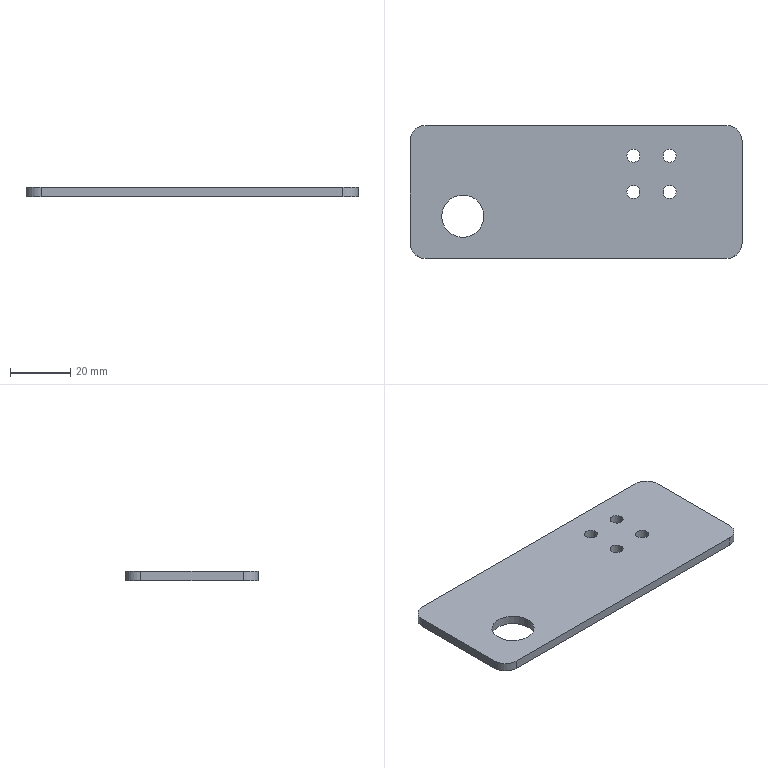Part | SolidWorks | features Fillet 2, Cut 1, Extrusion 1, ICE 1 | 1 solid | 20 faces | box 110 x 44 x 3 mm | volume 13820 mm3 | cylinder 14 | plane 6 | commonest cylinder face diameters 4.3 x8 10 x4 14 x2
STEP:
#1=CARTESIAN_POINT('',(-69.5,-8.,0.));
#2=VERTEX_POINT('',#1);
#3=CARTESIAN_POINT('',(-55.5,-8.,0.));
#4=VERTEX_POINT('',#3);
#5=CARTESIAN_POINT('',(-62.5,-8.,0.));
#6=DIRECTION('',(0.,0.,1.));
#7=DIRECTION('',(1.,0.,0.));
#8=AXIS2_PLACEMENT_3D('',#5,#6,#7);
#9=CIRCLE('',#8,7.);
#10=EDGE_CURVE('',#2,#4,#9,.T.);
#11=ORIENTED_EDGE('',*,*,#10,.F.);
#12=CARTESIAN_POINT('',(-69.5,-8.,3.));
#13=VERTEX_POINT('',#12);
#14=CARTESIAN_POINT('',(-69.5,-8.,0.));
#15=DIRECTION('',(0.,0.,1.));
#16=VECTOR('',#15,1000.);
#17=LINE('',#14,#16);
#18=EDGE_CURVE('',#2,#13,#17,.T.);
#19=ORIENTED_EDGE('',*,*,#18,.T.);
#20=CARTESIAN_POINT('',(-55.5,-8.,3.));
#21=VERTEX_POINT('',#20);
#22=CARTESIAN_POINT('',(-62.5,-8.,3.));
#23=DIRECTION('',(0.,0.,1.));
#24=DIRECTION('',(1.,0.,0.));
#25=AXIS2_PLACEMENT_3D('',#22,#23,#24);
#26=CIRCLE('',#25,7.);
#27=EDGE_CURVE('',#13,#21,#26,.T.);
#28=ORIENTED_EDGE('',*,*,#27,.T.);
#29=CARTESIAN_POINT('',(-55.5,-8.,0.));
#30=DIRECTION('',(0.,0.,1.));
#31=VECTOR('',#30,1000.);
#32=LINE('',#29,#31);
#33=EDGE_CURVE('',#4,#21,#32,.T.);
#34=ORIENTED_EDGE('',*,*,#33,.F.);
#35=EDGE_LOOP('',(#11,#19,#28,#34));
#36=FACE_OUTER_BOUND('',#35,.T.);
#37=CARTESIAN_POINT('',(-62.5,-8.,0.));
#38=DIRECTION('',(0.,0.,1.));
#39=DIRECTION('',(1.,0.,0.));
#40=AXIS2_PLACEMENT_3D('',#37,#38,#39);
#41=CYLINDRICAL_SURFACE('',#40,7.);
#42=ADVANCED_FACE('',(#36),#41,.F.);
#43=CARTESIAN_POINT('',(-8.15,0.,0.));
#44=VERTEX_POINT('',#43);
#45=CARTESIAN_POINT('',(-3.85,0.,0.));
#46=VERTEX_POINT('',#45);
#47=CARTESIAN_POINT('',(-6.,0.,0.));
#48=DIRECTION('',(0.,0.,1.));
#49=DIRECTION('',(1.,0.,0.));
#50=AXIS2_PLACEMENT_3D('',#47,#48,#49);
#51=CIRCLE('',#50,2.15);
#52=EDGE_CURVE('',#44,#46,#51,.T.);
#53=ORIENTED_EDGE('',*,*,#52,.F.);
#54=CARTESIAN_POINT('',(-8.15,0.,3.));
#55=VERTEX_POINT('',#54);
#56=CARTESIAN_POINT('',(-8.15,0.,0.));
#57=DIRECTION('',(0.,0.,1.));
#58=VECTOR('',#57,1000.);
#59=LINE('',#56,#58);
#60=EDGE_CURVE('',#44,#55,#59,.T.);
#61=ORIENTED_EDGE('',*,*,#60,.T.);
#62=CARTESIAN_POINT('',(-3.85,0.,3.));
#63=VERTEX_POINT('',#62);
#64=CARTESIAN_POINT('',(-6.,0.,3.));
#65=DIRECTION('',(0.,0.,1.));
#66=DIRECTION('',(1.,0.,0.));
#67=AXIS2_PLACEMENT_3D('',#64,#65,#66);
#68=CIRCLE('',#67,2.15);
#69=EDGE_CURVE('',#55,#63,#68,.T.);
#70=ORIENTED_EDGE('',*,*,#69,.T.);
#71=CARTESIAN_POINT('',(-3.85,0.,0.));
#72=DIRECTION('',(0.,0.,1.));
#73=VECTOR('',#72,1000.);
#74=LINE('',#71,#73);
#75=EDGE_CURVE('',#46,#63,#74,.T.);
#76=ORIENTED_EDGE('',*,*,#75,.F.);
#77=EDGE_LOOP('',(#53,#61,#70,#76));
#78=FACE_OUTER_BOUND('',#77,.T.);
#79=CARTESIAN_POINT('',(-6.,0.,0.));
#80=DIRECTION('',(0.,0.,1.));
#81=DIRECTION('',(1.,0.,0.));
#82=AXIS2_PLACEMENT_3D('',#79,#80,#81);
#83=CYLINDRICAL_SURFACE('',#82,2.15);
#84=ADVANCED_FACE('',(#78),#83,.F.);
#85=CARTESIAN_POINT('',(-8.15,12.,0.));
#86=VERTEX_POINT('',#85);
#87=CARTESIAN_POINT('',(-3.85,12.,0.));
#88=VERTEX_POINT('',#87);
#89=CARTESIAN_POINT('',(-6.,12.,0.));
#90=DIRECTION('',(0.,0.,1.));
#91=DIRECTION('',(1.,0.,0.));
#92=AXIS2_PLACEMENT_3D('',#89,#90,#91);
#93=CIRCLE('',#92,2.15);
#94=EDGE_CURVE('',#86,#88,#93,.T.);
#95=ORIENTED_EDGE('',*,*,#94,.F.);
#96=CARTESIAN_POINT('',(-8.15,12.,3.));
#97=VERTEX_POINT('',#96);
#98=CARTESIAN_POINT('',(-8.15,12.,0.));
#99=DIRECTION('',(0.,0.,1.));
#100=VECTOR('',#99,1000.);
#101=LINE('',#98,#100);
#102=EDGE_CURVE('',#86,#97,#101,.T.);
#103=ORIENTED_EDGE('',*,*,#102,.T.);
#104=CARTESIAN_POINT('',(-3.85,12.,3.));
#105=VERTEX_POINT('',#104);
#106=CARTESIAN_POINT('',(-6.,12.,3.));
#107=DIRECTION('',(0.,0.,1.));
#108=DIRECTION('',(1.,0.,0.));
#109=AXIS2_PLACEMENT_3D('',#106,#107,#108);
#110=CIRCLE('',#109,2.15);
#111=EDGE_CURVE('',#97,#105,#110,.T.);
#112=ORIENTED_EDGE('',*,*,#111,.T.);
#113=CARTESIAN_POINT('',(-3.85,12.,0.));
#114=DIRECTION('',(0.,0.,1.));
#115=VECTOR('',#114,1000.);
#116=LINE('',#113,#115);
#117=EDGE_CURVE('',#88,#105,#116,.T.);
#118=ORIENTED_EDGE('',*,*,#117,.F.);
#119=EDGE_LOOP('',(#95,#103,#112,#118));
#120=FACE_OUTER_BOUND('',#119,.T.);
#121=CARTESIAN_POINT('',(-6.,12.,0.));
#122=DIRECTION('',(0.,0.,1.));
#123=DIRECTION('',(1.,0.,0.));
#124=AXIS2_PLACEMENT_3D('',#121,#122,#123);
#125=CYLINDRICAL_SURFACE('',#124,2.15);
#126=ADVANCED_FACE('',(#120),#125,.F.);
#127=CARTESIAN_POINT('',(3.85,12.,0.));
#128=VERTEX_POINT('',#127);
#129=CARTESIAN_POINT('',(8.15,12.,0.));
#130=VERTEX_POINT('',#129);
#131=CARTESIAN_POINT('',(6.,12.,0.));
#132=DIRECTION('',(0.,0.,1.));
#133=DIRECTION('',(1.,0.,0.));
#134=AXIS2_PLACEMENT_3D('',#131,#132,#133);
#135=CIRCLE('',#134,2.15);
#136=EDGE_CURVE('',#128,#130,#135,.T.);
#137=ORIENTED_EDGE('',*,*,#136,.F.);
#138=CARTESIAN_POINT('',(3.85,12.,3.));
#139=VERTEX_POINT('',#138);
#140=CARTESIAN_POINT('',(3.85,12.,0.));
#141=DIRECTION('',(0.,0.,1.));
#142=VECTOR('',#141,1000.);
#143=LINE('',#140,#142);
#144=EDGE_CURVE('',#128,#139,#143,.T.);
#145=ORIENTED_EDGE('',*,*,#144,.T.);
#146=CARTESIAN_POINT('',(8.15,12.,3.));
#147=VERTEX_POINT('',#146);
#148=CARTESIAN_POINT('',(6.,12.,3.));
#149=DIRECTION('',(0.,0.,1.));
#150=DIRECTION('',(1.,0.,0.));
#151=AXIS2_PLACEMENT_3D('',#148,#149,#150);
#152=CIRCLE('',#151,2.15);
#153=EDGE_CURVE('',#139,#147,#152,.T.);
#154=ORIENTED_EDGE('',*,*,#153,.T.);
#155=CARTESIAN_POINT('',(8.15,12.,0.));
#156=DIRECTION('',(0.,0.,1.));
#157=VECTOR('',#156,1000.);
#158=LINE('',#155,#157);
#159=EDGE_CURVE('',#130,#147,#158,.T.);
#160=ORIENTED_EDGE('',*,*,#159,.F.);
#161=EDGE_LOOP('',(#137,#145,#154,#160));
#162=FACE_OUTER_BOUND('',#161,.T.);
#163=CARTESIAN_POINT('',(6.,12.,0.));
#164=DIRECTION('',(0.,0.,1.));
#165=DIRECTION('',(1.,0.,0.));
#166=AXIS2_PLACEMENT_3D('',#163,#164,#165);
#167=CYLINDRICAL_SURFACE('',#166,2.15);
#168=ADVANCED_FACE('',(#162),#167,.F.);
#169=CARTESIAN_POINT('',(3.85,0.,0.));
#170=VERTEX_POINT('',#169);
#171=CARTESIAN_POINT('',(8.15,0.,0.));
#172=VERTEX_POINT('',#171);
#173=CARTESIAN_POINT('',(6.,0.,0.));
#174=DIRECTION('',(0.,0.,1.));
#175=DIRECTION('',(1.,0.,0.));
#176=AXIS2_PLACEMENT_3D('',#173,#174,#175);
#177=CIRCLE('',#176,2.15);
#178=EDGE_CURVE('',#170,#172,#177,.T.);
#179=ORIENTED_EDGE('',*,*,#178,.F.);
#180=CARTESIAN_POINT('',(3.85,0.,3.));
#181=VERTEX_POINT('',#180);
#182=CARTESIAN_POINT('',(3.85,0.,0.));
#183=DIRECTION('',(0.,0.,1.));
#184=VECTOR('',#183,1000.);
#185=LINE('',#182,#184);
#186=EDGE_CURVE('',#170,#181,#185,.T.);
#187=ORIENTED_EDGE('',*,*,#186,.T.);
#188=CARTESIAN_POINT('',(8.15,0.,3.));
#189=VERTEX_POINT('',#188);
#190=CARTESIAN_POINT('',(6.,0.,3.));
#191=DIRECTION('',(0.,0.,1.));
#192=DIRECTION('',(1.,0.,0.));
#193=AXIS2_PLACEMENT_3D('',#190,#191,#192);
#194=CIRCLE('',#193,2.15);
#195=EDGE_CURVE('',#181,#189,#194,.T.);
#196=ORIENTED_EDGE('',*,*,#195,.T.);
#197=CARTESIAN_POINT('',(8.15,0.,0.));
#198=DIRECTION('',(0.,0.,1.));
#199=VECTOR('',#198,1000.);
#200=LINE('',#197,#199);
#201=EDGE_CURVE('',#172,#189,#200,.T.);
#202=ORIENTED_EDGE('',*,*,#201,.F.);
#203=EDGE_LOOP('',(#179,#187,#196,#202));
#204=FACE_OUTER_BOUND('',#203,.T.);
#205=CARTESIAN_POINT('',(6.,0.,0.));
#206=DIRECTION('',(0.,0.,1.));
#207=DIRECTION('',(1.,0.,0.));
#208=AXIS2_PLACEMENT_3D('',#205,#206,#207);
#209=CYLINDRICAL_SURFACE('',#208,2.15);
#210=ADVANCED_FACE('',(#204),#209,.F.);
#211=CARTESIAN_POINT('',(25.,22.,3.));
#212=VERTEX_POINT('',#211);
#213=CARTESIAN_POINT('',(-75.,22.,3.));
#214=VERTEX_POINT('',#213);
#215=CARTESIAN_POINT('',(-80.,22.,3.));
#216=DIRECTION('',(-1.,0.,0.));
#217=VECTOR('',#216,1000.);
#218=LINE('',#215,#217);
#219=EDGE_CURVE('',#212,#214,#218,.T.);
#220=ORIENTED_EDGE('',*,*,#219,.F.);
#221=CARTESIAN_POINT('',(25.,22.,0.));
#222=VERTEX_POINT('',#221);
#223=CARTESIAN_POINT('',(25.,22.,3.));
#224=DIRECTION('',(0.,0.,-1.));
#225=VECTOR('',#224,1000.);
#226=LINE('',#223,#225);
#227=EDGE_CURVE('',#212,#222,#226,.T.);
#228=ORIENTED_EDGE('',*,*,#227,.T.);
#229=CARTESIAN_POINT('',(-75.,22.,0.));
#230=VERTEX_POINT('',#229);
#231=CARTESIAN_POINT('',(-80.,22.,0.));
#232=DIRECTION('',(-1.,0.,0.));
#233=VECTOR('',#232,1000.);
#234=LINE('',#231,#233);
#235=EDGE_CURVE('',#222,#230,#234,.T.);
#236=ORIENTED_EDGE('',*,*,#235,.T.);
#237=CARTESIAN_POINT('',(-75.,22.,3.));
#238=DIRECTION('',(0.,0.,1.));
#239=VECTOR('',#238,1000.);
#240=LINE('',#237,#239);
#241=EDGE_CURVE('',#230,#214,#240,.T.);
#242=ORIENTED_EDGE('',*,*,#241,.T.);
#243=EDGE_LOOP('',(#220,#228,#236,#242));
#244=FACE_OUTER_BOUND('',#243,.T.);
#245=CARTESIAN_POINT('',(-80.,22.,3.));
#246=DIRECTION('',(0.,-1.,0.));
#247=DIRECTION('',(0.,0.,-1.));
#248=AXIS2_PLACEMENT_3D('',#245,#246,#247);
#249=PLANE('',#248);
#250=ADVANCED_FACE('',(#244),#249,.F.);
#251=CARTESIAN_POINT('',(-80.,17.,3.));
#252=VERTEX_POINT('',#251);
#253=CARTESIAN_POINT('',(-80.,-17.,3.));
#254=VERTEX_POINT('',#253);
#255=CARTESIAN_POINT('',(-80.,22.,3.));
#256=DIRECTION('',(0.,-1.,0.));
#257=VECTOR('',#256,1000.);
#258=LINE('',#255,#257);
#259=EDGE_CURVE('',#252,#254,#258,.T.);
#260=ORIENTED_EDGE('',*,*,#259,.F.);
#261=CARTESIAN_POINT('',(-80.,17.,0.));
#262=VERTEX_POINT('',#261);
#263=CARTESIAN_POINT('',(-80.,17.,3.));
#264=DIRECTION('',(0.,0.,-1.));
#265=VECTOR('',#264,1000.);
#266=LINE('',#263,#265);
#267=EDGE_CURVE('',#252,#262,#266,.T.);
#268=ORIENTED_EDGE('',*,*,#267,.T.);
#269=CARTESIAN_POINT('',(-80.,-17.,0.));
#270=VERTEX_POINT('',#269);
#271=CARTESIAN_POINT('',(-80.,22.,0.));
#272=DIRECTION('',(0.,-1.,0.));
#273=VECTOR('',#272,1000.);
#274=LINE('',#271,#273);
#275=EDGE_CURVE('',#262,#270,#274,.T.);
#276=ORIENTED_EDGE('',*,*,#275,.T.);
#277=CARTESIAN_POINT('',(-80.,-17.,3.));
#278=DIRECTION('',(0.,0.,1.));
#279=VECTOR('',#278,1000.);
#280=LINE('',#277,#279);
#281=EDGE_CURVE('',#270,#254,#280,.T.);
#282=ORIENTED_EDGE('',*,*,#281,.T.);
#283=EDGE_LOOP('',(#260,#268,#276,#282));
#284=FACE_OUTER_BOUND('',#283,.T.);
#285=CARTESIAN_POINT('',(-80.,22.,3.));
#286=DIRECTION('',(1.,0.,0.));
#287=DIRECTION('',(0.,0.,-1.));
#288=AXIS2_PLACEMENT_3D('',#285,#286,#287);
#289=PLANE('',#288);
#290=ADVANCED_FACE('',(#284),#289,.F.);
#291=CARTESIAN_POINT('',(-75.,-22.,0.));
#292=VERTEX_POINT('',#291);
#293=CARTESIAN_POINT('',(25.,-22.,0.));
#294=VERTEX_POINT('',#293);
#295=CARTESIAN_POINT('',(-80.,-22.,0.));
#296=DIRECTION('',(1.,0.,0.));
#297=VECTOR('',#296,1000.);
#298=LINE('',#295,#297);
#299=EDGE_CURVE('',#292,#294,#298,.T.);
#300=ORIENTED_EDGE('',*,*,#299,.T.);
#301=CARTESIAN_POINT('',(25.,-22.,3.));
#302=VERTEX_POINT('',#301);
#303=CARTESIAN_POINT('',(25.,-22.,3.));
#304=DIRECTION('',(0.,0.,1.));
#305=VECTOR('',#304,1000.);
#306=LINE('',#303,#305);
#307=EDGE_CURVE('',#294,#302,#306,.T.);
#308=ORIENTED_EDGE('',*,*,#307,.T.);
#309=CARTESIAN_POINT('',(-75.,-22.,3.));
#310=VERTEX_POINT('',#309);
#311=CARTESIAN_POINT('',(-80.,-22.,3.));
#312=DIRECTION('',(1.,0.,0.));
#313=VECTOR('',#312,1000.);
#314=LINE('',#311,#313);
#315=EDGE_CURVE('',#310,#302,#314,.T.);
#316=ORIENTED_EDGE('',*,*,#315,.F.);
#317=CARTESIAN_POINT('',(-75.,-22.,3.));
#318=DIRECTION('',(0.,0.,-1.));
#319=VECTOR('',#318,1000.);
#320=LINE('',#317,#319);
#321=EDGE_CURVE('',#310,#292,#320,.T.);
#322=ORIENTED_EDGE('',*,*,#321,.T.);
#323=EDGE_LOOP('',(#300,#308,#316,#322));
#324=FACE_OUTER_BOUND('',#323,.T.);
#325=CARTESIAN_POINT('',(-80.,-22.,3.));
#326=DIRECTION('',(0.,1.,0.));
#327=DIRECTION('',(0.,0.,1.));
#328=AXIS2_PLACEMENT_3D('',#325,#326,#327);
#329=PLANE('',#328);
#330=ADVANCED_FACE('',(#324),#329,.F.);
#331=ORIENTED_EDGE('',*,*,#315,.T.);
#332=CARTESIAN_POINT('',(30.,-17.,3.));
#333=VERTEX_POINT('',#332);
#334=CARTESIAN_POINT('',(25.,-17.,3.));
#335=DIRECTION('',(0.,0.,1.));
#336=DIRECTION('',(1.,0.,0.));
#337=AXIS2_PLACEMENT_3D('',#334,#335,#336);
#338=CIRCLE('',#337,5.);
#339=EDGE_CURVE('',#302,#333,#338,.T.);
#340=ORIENTED_EDGE('',*,*,#339,.T.);
#341=CARTESIAN_POINT('',(30.,17.,3.));
#342=VERTEX_POINT('',#341);
#343=CARTESIAN_POINT('',(30.,-36.164,3.));
#344=DIRECTION('',(0.,-1.,0.));
#345=VECTOR('',#344,1000.);
#346=LINE('',#343,#345);
#347=EDGE_CURVE('',#342,#333,#346,.T.);
#348=ORIENTED_EDGE('',*,*,#347,.F.);
#349=CARTESIAN_POINT('',(25.,17.,3.));
#350=DIRECTION('',(0.,0.,1.));
#351=DIRECTION('',(1.,0.,0.));
#352=AXIS2_PLACEMENT_3D('',#349,#350,#351);
#353=CIRCLE('',#352,5.);
#354=EDGE_CURVE('',#342,#212,#353,.T.);
#355=ORIENTED_EDGE('',*,*,#354,.T.);
#356=ORIENTED_EDGE('',*,*,#219,.T.);
#357=CARTESIAN_POINT('',(-75.,17.,3.));
#358=DIRECTION('',(0.,0.,1.));
#359=DIRECTION('',(1.,0.,0.));
#360=AXIS2_PLACEMENT_3D('',#357,#358,#359);
#361=CIRCLE('',#360,5.);
#362=EDGE_CURVE('',#214,#252,#361,.T.);
#363=ORIENTED_EDGE('',*,*,#362,.T.);
#364=ORIENTED_EDGE('',*,*,#259,.T.);
#365=CARTESIAN_POINT('',(-75.,-17.,3.));
#366=DIRECTION('',(0.,0.,1.));
#367=DIRECTION('',(1.,0.,0.));
#368=AXIS2_PLACEMENT_3D('',#365,#366,#367);
#369=CIRCLE('',#368,5.);
#370=EDGE_CURVE('',#254,#310,#369,.T.);
#371=ORIENTED_EDGE('',*,*,#370,.T.);
#372=EDGE_LOOP('',(#331,#340,#348,#355,#356,#363,#364,#371));
#373=FACE_OUTER_BOUND('',#372,.T.);
#374=CARTESIAN_POINT('',(-62.5,-8.,3.));
#375=DIRECTION('',(0.,0.,1.));
#376=DIRECTION('',(1.,0.,0.));
#377=AXIS2_PLACEMENT_3D('',#374,#375,#376);
#378=CIRCLE('',#377,7.);
#379=EDGE_CURVE('',#21,#13,#378,.T.);
#380=ORIENTED_EDGE('',*,*,#379,.F.);
#381=ORIENTED_EDGE('',*,*,#27,.F.);
#382=EDGE_LOOP('',(#380,#381));
#383=FACE_BOUND('',#382,.T.);
#384=CARTESIAN_POINT('',(-6.,0.,3.));
#385=DIRECTION('',(0.,0.,1.));
#386=DIRECTION('',(1.,0.,0.));
#387=AXIS2_PLACEMENT_3D('',#384,#385,#386);
#388=CIRCLE('',#387,2.15);
#389=EDGE_CURVE('',#63,#55,#388,.T.);
#390=ORIENTED_EDGE('',*,*,#389,.F.);
#391=ORIENTED_EDGE('',*,*,#69,.F.);
#392=EDGE_LOOP('',(#390,#391));
#393=FACE_BOUND('',#392,.T.);
#394=CARTESIAN_POINT('',(-6.,12.,3.));
#395=DIRECTION('',(0.,0.,1.));
#396=DIRECTION('',(1.,0.,0.));
#397=AXIS2_PLACEMENT_3D('',#394,#395,#396);
#398=CIRCLE('',#397,2.15);
#399=EDGE_CURVE('',#105,#97,#398,.T.);
#400=ORIENTED_EDGE('',*,*,#399,.F.);
#401=ORIENTED_EDGE('',*,*,#111,.F.);
#402=EDGE_LOOP('',(#400,#401));
#403=FACE_BOUND('',#402,.T.);
#404=CARTESIAN_POINT('',(6.,12.,3.));
#405=DIRECTION('',(0.,0.,1.));
#406=DIRECTION('',(1.,0.,0.));
#407=AXIS2_PLACEMENT_3D('',#404,#405,#406);
#408=CIRCLE('',#407,2.15);
#409=EDGE_CURVE('',#147,#139,#408,.T.);
#410=ORIENTED_EDGE('',*,*,#409,.F.);
#411=ORIENTED_EDGE('',*,*,#153,.F.);
#412=EDGE_LOOP('',(#410,#411));
#413=FACE_BOUND('',#412,.T.);
#414=CARTESIAN_POINT('',(6.,0.,3.));
#415=DIRECTION('',(0.,0.,1.));
#416=DIRECTION('',(1.,0.,0.));
#417=AXIS2_PLACEMENT_3D('',#414,#415,#416);
#418=CIRCLE('',#417,2.15);
#419=EDGE_CURVE('',#189,#181,#418,.T.);
#420=ORIENTED_EDGE('',*,*,#419,.F.);
#421=ORIENTED_EDGE('',*,*,#195,.F.);
#422=EDGE_LOOP('',(#420,#421));
#423=FACE_BOUND('',#422,.T.);
#424=CARTESIAN_POINT('',(0.,0.,3.));
#425=DIRECTION('',(0.,0.,1.));
#426=DIRECTION('',(1.,0.,0.));
#427=AXIS2_PLACEMENT_3D('',#424,#425,#426);
#428=PLANE('',#427);
#429=ADVANCED_FACE('',(#373,#383,#393,#403,#413,#423),#428,.T.);
#430=CARTESIAN_POINT('',(-62.5,-8.,0.));
#431=DIRECTION('',(0.,0.,1.));
#432=DIRECTION('',(1.,0.,0.));
#433=AXIS2_PLACEMENT_3D('',#430,#431,#432);
#434=CIRCLE('',#433,7.);
#435=EDGE_CURVE('',#4,#2,#434,.T.);
#436=ORIENTED_EDGE('',*,*,#435,.T.);
#437=ORIENTED_EDGE('',*,*,#10,.T.);
#438=EDGE_LOOP('',(#436,#437));
#439=FACE_BOUND('',#438,.T.);
#440=CARTESIAN_POINT('',(-6.,0.,0.));
#441=DIRECTION('',(0.,0.,1.));
#442=DIRECTION('',(1.,0.,0.));
#443=AXIS2_PLACEMENT_3D('',#440,#441,#442);
#444=CIRCLE('',#443,2.15);
#445=EDGE_CURVE('',#46,#44,#444,.T.);
#446=ORIENTED_EDGE('',*,*,#445,.T.);
#447=ORIENTED_EDGE('',*,*,#52,.T.);
#448=EDGE_LOOP('',(#446,#447));
#449=FACE_BOUND('',#448,.T.);
#450=CARTESIAN_POINT('',(-6.,12.,0.));
#451=DIRECTION('',(0.,0.,1.));
#452=DIRECTION('',(1.,0.,0.));
#453=AXIS2_PLACEMENT_3D('',#450,#451,#452);
#454=CIRCLE('',#453,2.15);
#455=EDGE_CURVE('',#88,#86,#454,.T.);
#456=ORIENTED_EDGE('',*,*,#455,.T.);
#457=ORIENTED_EDGE('',*,*,#94,.T.);
#458=EDGE_LOOP('',(#456,#457));
#459=FACE_BOUND('',#458,.T.);
#460=CARTESIAN_POINT('',(6.,12.,0.));
#461=DIRECTION('',(0.,0.,1.));
#462=DIRECTION('',(1.,0.,0.));
#463=AXIS2_PLACEMENT_3D('',#460,#461,#462);
#464=CIRCLE('',#463,2.15);
#465=EDGE_CURVE('',#130,#128,#464,.T.);
#466=ORIENTED_EDGE('',*,*,#465,.T.);
#467=ORIENTED_EDGE('',*,*,#136,.T.);
#468=EDGE_LOOP('',(#466,#467));
#469=FACE_BOUND('',#468,.T.);
#470=CARTESIAN_POINT('',(6.,0.,0.));
#471=DIRECTION('',(0.,0.,1.));
#472=DIRECTION('',(1.,0.,0.));
#473=AXIS2_PLACEMENT_3D('',#470,#471,#472);
#474=CIRCLE('',#473,2.15);
#475=EDGE_CURVE('',#172,#170,#474,.T.);
#476=ORIENTED_EDGE('',*,*,#475,.T.);
#477=ORIENTED_EDGE('',*,*,#178,.T.);
#478=EDGE_LOOP('',(#476,#477));
#479=FACE_BOUND('',#478,.T.);
#480=CARTESIAN_POINT('',(30.,17.,0.));
#481=VERTEX_POINT('',#480);
#482=CARTESIAN_POINT('',(30.,-17.,0.));
#483=VERTEX_POINT('',#482);
#484=CARTESIAN_POINT('',(30.,0.,0.));
#485=DIRECTION('',(0.,-1.,0.));
#486=VECTOR('',#485,1000.);
#487=LINE('',#484,#486);
#488=EDGE_CURVE('',#481,#483,#487,.T.);
#489=ORIENTED_EDGE('',*,*,#488,.T.);
#490=CARTESIAN_POINT('',(25.,-17.,0.));
#491=DIRECTION('',(0.,0.,-1.));
#492=DIRECTION('',(1.,0.,0.));
#493=AXIS2_PLACEMENT_3D('',#490,#491,#492);
#494=CIRCLE('',#493,5.);
#495=EDGE_CURVE('',#483,#294,#494,.T.);
#496=ORIENTED_EDGE('',*,*,#495,.T.);
#497=ORIENTED_EDGE('',*,*,#299,.F.);
#498=CARTESIAN_POINT('',(-75.,-17.,0.));
#499=DIRECTION('',(0.,0.,-1.));
#500=DIRECTION('',(1.,0.,0.));
#501=AXIS2_PLACEMENT_3D('',#498,#499,#500);
#502=CIRCLE('',#501,5.);
#503=EDGE_CURVE('',#292,#270,#502,.T.);
#504=ORIENTED_EDGE('',*,*,#503,.T.);
#505=ORIENTED_EDGE('',*,*,#275,.F.);
#506=CARTESIAN_POINT('',(-75.,17.,0.));
#507=DIRECTION('',(0.,0.,-1.));
#508=DIRECTION('',(1.,0.,0.));
#509=AXIS2_PLACEMENT_3D('',#506,#507,#508);
#510=CIRCLE('',#509,5.);
#511=EDGE_CURVE('',#262,#230,#510,.T.);
#512=ORIENTED_EDGE('',*,*,#511,.T.);
#513=ORIENTED_EDGE('',*,*,#235,.F.);
#514=CARTESIAN_POINT('',(25.,17.,0.));
#515=DIRECTION('',(0.,0.,-1.));
#516=DIRECTION('',(1.,0.,0.));
#517=AXIS2_PLACEMENT_3D('',#514,#515,#516);
#518=CIRCLE('',#517,5.);
#519=EDGE_CURVE('',#222,#481,#518,.T.);
#520=ORIENTED_EDGE('',*,*,#519,.T.);
#521=EDGE_LOOP('',(#489,#496,#497,#504,#505,#512,#513,#520));
#522=FACE_OUTER_BOUND('',#521,.T.);
#523=CARTESIAN_POINT('',(0.,0.,0.));
#524=DIRECTION('',(0.,0.,1.));
#525=DIRECTION('',(1.,0.,0.));
#526=AXIS2_PLACEMENT_3D('',#523,#524,#525);
#527=PLANE('',#526);
#528=ADVANCED_FACE('',(#439,#449,#459,#469,#479,#522),#527,.F.);
#529=ORIENTED_EDGE('',*,*,#186,.F.);
#530=ORIENTED_EDGE('',*,*,#475,.F.);
#531=ORIENTED_EDGE('',*,*,#201,.T.);
#532=ORIENTED_EDGE('',*,*,#419,.T.);
#533=EDGE_LOOP('',(#529,#530,#531,#532));
#534=FACE_OUTER_BOUND('',#533,.T.);
#535=CARTESIAN_POINT('',(6.,0.,0.));
#536=DIRECTION('',(0.,0.,1.));
#537=DIRECTION('',(1.,0.,0.));
#538=AXIS2_PLACEMENT_3D('',#535,#536,#537);
#539=CYLINDRICAL_SURFACE('',#538,2.15);
#540=ADVANCED_FACE('',(#534),#539,.F.);
#541=ORIENTED_EDGE('',*,*,#144,.F.);
#542=ORIENTED_EDGE('',*,*,#465,.F.);
#543=ORIENTED_EDGE('',*,*,#159,.T.);
#544=ORIENTED_EDGE('',*,*,#409,.T.);
#545=EDGE_LOOP('',(#541,#542,#543,#544));
#546=FACE_OUTER_BOUND('',#545,.T.);
#547=CARTESIAN_POINT('',(6.,12.,0.));
#548=DIRECTION('',(0.,0.,1.));
#549=DIRECTION('',(1.,0.,0.));
#550=AXIS2_PLACEMENT_3D('',#547,#548,#549);
#551=CYLINDRICAL_SURFACE('',#550,2.15);
#552=ADVANCED_FACE('',(#546),#551,.F.);
#553=ORIENTED_EDGE('',*,*,#102,.F.);
#554=ORIENTED_EDGE('',*,*,#455,.F.);
#555=ORIENTED_EDGE('',*,*,#117,.T.);
#556=ORIENTED_EDGE('',*,*,#399,.T.);
#557=EDGE_LOOP('',(#553,#554,#555,#556));
#558=FACE_OUTER_BOUND('',#557,.T.);
#559=CARTESIAN_POINT('',(-6.,12.,0.));
#560=DIRECTION('',(0.,0.,1.));
#561=DIRECTION('',(1.,0.,0.));
#562=AXIS2_PLACEMENT_3D('',#559,#560,#561);
#563=CYLINDRICAL_SURFACE('',#562,2.15);
#564=ADVANCED_FACE('',(#558),#563,.F.);
#565=ORIENTED_EDGE('',*,*,#60,.F.);
#566=ORIENTED_EDGE('',*,*,#445,.F.);
#567=ORIENTED_EDGE('',*,*,#75,.T.);
#568=ORIENTED_EDGE('',*,*,#389,.T.);
#569=EDGE_LOOP('',(#565,#566,#567,#568));
#570=FACE_OUTER_BOUND('',#569,.T.);
#571=CARTESIAN_POINT('',(-6.,0.,0.));
#572=DIRECTION('',(0.,0.,1.));
#573=DIRECTION('',(1.,0.,0.));
#574=AXIS2_PLACEMENT_3D('',#571,#572,#573);
#575=CYLINDRICAL_SURFACE('',#574,2.15);
#576=ADVANCED_FACE('',(#570),#575,.F.);
#577=ORIENTED_EDGE('',*,*,#18,.F.);
#578=ORIENTED_EDGE('',*,*,#435,.F.);
#579=ORIENTED_EDGE('',*,*,#33,.T.);
#580=ORIENTED_EDGE('',*,*,#379,.T.);
#581=EDGE_LOOP('',(#577,#578,#579,#580));
#582=FACE_OUTER_BOUND('',#581,.T.);
#583=CARTESIAN_POINT('',(-62.5,-8.,0.));
#584=DIRECTION('',(0.,0.,1.));
#585=DIRECTION('',(1.,0.,0.));
#586=AXIS2_PLACEMENT_3D('',#583,#584,#585);
#587=CYLINDRICAL_SURFACE('',#586,7.);
#588=ADVANCED_FACE('',(#582),#587,.F.);
#589=ORIENTED_EDGE('',*,*,#362,.F.);
#590=ORIENTED_EDGE('',*,*,#241,.F.);
#591=ORIENTED_EDGE('',*,*,#511,.F.);
#592=ORIENTED_EDGE('',*,*,#267,.F.);
#593=EDGE_LOOP('',(#589,#590,#591,#592));
#594=FACE_OUTER_BOUND('',#593,.T.);
#595=CARTESIAN_POINT('',(-75.,17.,3.));
#596=DIRECTION('',(0.,0.,-1.));
#597=DIRECTION('',(-1.,0.,0.));
#598=AXIS2_PLACEMENT_3D('',#595,#596,#597);
#599=CYLINDRICAL_SURFACE('',#598,5.);
#600=ADVANCED_FACE('',(#594),#599,.T.);
#601=ORIENTED_EDGE('',*,*,#370,.F.);
#602=ORIENTED_EDGE('',*,*,#281,.F.);
#603=ORIENTED_EDGE('',*,*,#503,.F.);
#604=ORIENTED_EDGE('',*,*,#321,.F.);
#605=EDGE_LOOP('',(#601,#602,#603,#604));
#606=FACE_OUTER_BOUND('',#605,.T.);
#607=CARTESIAN_POINT('',(-75.,-17.,3.));
#608=DIRECTION('',(0.,0.,-1.));
#609=DIRECTION('',(-1.,0.,0.));
#610=AXIS2_PLACEMENT_3D('',#607,#608,#609);
#611=CYLINDRICAL_SURFACE('',#610,5.);
#612=ADVANCED_FACE('',(#606),#611,.T.);
#613=ORIENTED_EDGE('',*,*,#347,.T.);
#614=CARTESIAN_POINT('',(30.,-17.,-7.));
#615=DIRECTION('',(0.,0.,-1.));
#616=VECTOR('',#615,1000.);
#617=LINE('',#614,#616);
#618=EDGE_CURVE('',#333,#483,#617,.T.);
#619=ORIENTED_EDGE('',*,*,#618,.T.);
#620=ORIENTED_EDGE('',*,*,#488,.F.);
#621=CARTESIAN_POINT('',(30.,17.,-7.));
#622=DIRECTION('',(0.,0.,1.));
#623=VECTOR('',#622,1000.);
#624=LINE('',#621,#623);
#625=EDGE_CURVE('',#481,#342,#624,.T.);
#626=ORIENTED_EDGE('',*,*,#625,.T.);
#627=EDGE_LOOP('',(#613,#619,#620,#626));
#628=FACE_OUTER_BOUND('',#627,.T.);
#629=CARTESIAN_POINT('',(30.,-36.164,-7.));
#630=DIRECTION('',(-1.,0.,0.));
#631=DIRECTION('',(0.,0.,1.));
#632=AXIS2_PLACEMENT_3D('',#629,#630,#631);
#633=PLANE('',#632);
#634=ADVANCED_FACE('',(#628),#633,.F.);
#635=ORIENTED_EDGE('',*,*,#495,.F.);
#636=ORIENTED_EDGE('',*,*,#618,.F.);
#637=ORIENTED_EDGE('',*,*,#339,.F.);
#638=ORIENTED_EDGE('',*,*,#307,.F.);
#639=EDGE_LOOP('',(#635,#636,#637,#638));
#640=FACE_OUTER_BOUND('',#639,.T.);
#641=CARTESIAN_POINT('',(25.,-17.,3.));
#642=DIRECTION('',(0.,0.,1.));
#643=DIRECTION('',(1.,0.,0.));
#644=AXIS2_PLACEMENT_3D('',#641,#642,#643);
#645=CYLINDRICAL_SURFACE('',#644,5.);
#646=ADVANCED_FACE('',(#640),#645,.T.);
#647=ORIENTED_EDGE('',*,*,#354,.F.);
#648=ORIENTED_EDGE('',*,*,#625,.F.);
#649=ORIENTED_EDGE('',*,*,#519,.F.);
#650=ORIENTED_EDGE('',*,*,#227,.F.);
#651=EDGE_LOOP('',(#647,#648,#649,#650));
#652=FACE_OUTER_BOUND('',#651,.T.);
#653=CARTESIAN_POINT('',(25.,17.,3.));
#654=DIRECTION('',(0.,0.,-1.));
#655=DIRECTION('',(-1.,0.,0.));
#656=AXIS2_PLACEMENT_3D('',#653,#654,#655);
#657=CYLINDRICAL_SURFACE('',#656,5.);
#658=ADVANCED_FACE('',(#652),#657,.T.);
#659=CLOSED_SHELL('',(#42,#84,#126,#168,#210,#250,#290,#330,#429,#528,#540,#552,#564,#576,#588,#600,#612,#634,#646,#658));
#660=MANIFOLD_SOLID_BREP('',#659);
#661=CARTESIAN_POINT('',(0.,0.,0.));
#662=DIRECTION('',(0.,0.,1.));
#663=DIRECTION('',(1.,0.,0.));
#664=AXIS2_PLACEMENT_3D('',#661,#662,#663);
#665=(LENGTH_UNIT()NAMED_UNIT(*)SI_UNIT(.MILLI.,.METRE.));
#666=UNCERTAINTY_MEASURE_WITH_UNIT(LENGTH_MEASURE(0.00001),#665,'','');
#667=(NAMED_UNIT(*)PLANE_ANGLE_UNIT()SI_UNIT($,.RADIAN.));
#668=(NAMED_UNIT(*)SI_UNIT($,.STERADIAN.)SOLID_ANGLE_UNIT());
#669=(GEOMETRIC_REPRESENTATION_CONTEXT(3)GLOBAL_UNCERTAINTY_ASSIGNED_CONTEXT((#666))GLOBAL_UNIT_ASSIGNED_CONTEXT((#665,#667,#668))REPRESENTATION_CONTEXT('',''));
#670=ADVANCED_BREP_SHAPE_REPRESENTATION('',(#660,#664),#669);